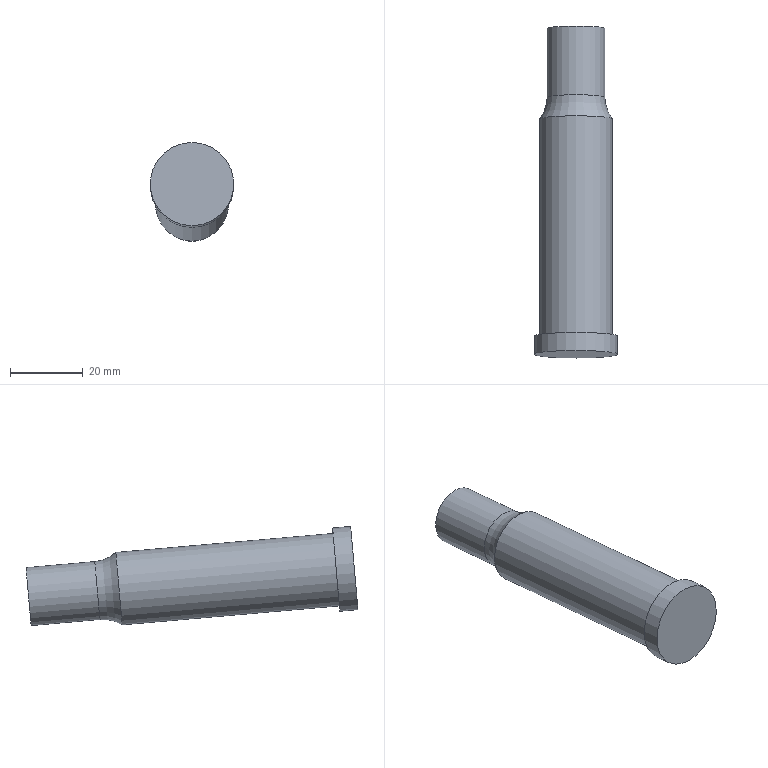Part | NX | features SPAS 20-80-16.00 2 | 1 solid | 7 faces | box 23 x 91.357 x 27.27 mm | volume 26160 mm3 | plane 3 | cylinder 3 | torus 1 | commonest cylinder face diameters 16 x1 20 x1 23 x1
STEP:
#1=CARTESIAN_POINT('',(398.525,-58.243,-48.565));
#2=VERTEX_POINT('',#1);
#3=CARTESIAN_POINT('',(398.525,-57.546,-40.595));
#4=DIRECTION('',(0.,-0.9962,0.08716));
#5=DIRECTION('',(0.,-0.08716,-0.9962));
#6=AXIS2_PLACEMENT_3D('',#3,#4,#5);
#7=CIRCLE('',#6,8.);
#8=EDGE_CURVE('',#2,#2,#7,.T.);
#9=ORIENTED_EDGE('',*,*,#8,.F.);
#10=EDGE_LOOP('',(#9));
#11=FACE_BOUND('',#10,.T.);
#12=CARTESIAN_POINT('',(398.525,-57.546,-40.595));
#13=DIRECTION('',(0.,0.9962,-0.08716));
#14=DIRECTION('',(0.,0.08716,0.9962));
#15=AXIS2_PLACEMENT_3D('',#12,#13,#14);
#16=PLANE('',#15);
#17=ADVANCED_FACE('',(#11),#16,.T.);
#18=CARTESIAN_POINT('',(398.525,-77.171,-46.909));
#19=VERTEX_POINT('',#18);
#20=CARTESIAN_POINT('',(398.525,-76.474,-38.939));
#21=DIRECTION('',(0.,-0.9962,0.08716));
#22=DIRECTION('',(0.,-0.08716,-0.9962));
#23=AXIS2_PLACEMENT_3D('',#20,#21,#22);
#24=CIRCLE('',#23,8.);
#25=EDGE_CURVE('',#19,#19,#24,.F.);
#26=ORIENTED_EDGE('',*,*,#25,.T.);
#27=EDGE_LOOP('',(#26));
#28=FACE_BOUND('',#27,.T.);
#29=ORIENTED_EDGE('',*,*,#8,.T.);
#30=EDGE_LOOP('',(#29));
#31=FACE_BOUND('',#30,.T.);
#32=CARTESIAN_POINT('',(398.525,-57.546,-40.595));
#33=DIRECTION('',(0.,-0.9962,0.08716));
#34=DIRECTION('',(0.,-0.08716,-0.9962));
#35=AXIS2_PLACEMENT_3D('',#32,#33,#34);
#36=CYLINDRICAL_SURFACE('',#35,8.);
#37=ADVANCED_FACE('',(#28,#31),#36,.T.);
#38=CARTESIAN_POINT('',(398.525,-141.351,-23.225));
#39=VERTEX_POINT('',#38);
#40=CARTESIAN_POINT('',(398.525,-142.222,-33.187));
#41=DIRECTION('',(0.,0.9962,-0.08716));
#42=DIRECTION('',(0.,0.08716,0.9962));
#43=AXIS2_PLACEMENT_3D('',#40,#41,#42);
#44=CIRCLE('',#43,10.);
#45=EDGE_CURVE('',#39,#39,#44,.F.);
#46=ORIENTED_EDGE('',*,*,#45,.F.);
#47=EDGE_LOOP('',(#46));
#48=FACE_BOUND('',#47,.T.);
#49=CARTESIAN_POINT('',(398.525,-83.322,-48.378));
#50=VERTEX_POINT('',#49);
#51=CARTESIAN_POINT('',(398.525,-82.451,-38.416));
#52=DIRECTION('',(0.,-0.9962,0.08716));
#53=DIRECTION('',(0.,-0.08716,-0.9962));
#54=AXIS2_PLACEMENT_3D('',#51,#52,#53);
#55=CIRCLE('',#54,10.);
#56=EDGE_CURVE('',#50,#50,#55,.T.);
#57=ORIENTED_EDGE('',*,*,#56,.T.);
#58=EDGE_LOOP('',(#57));
#59=FACE_BOUND('',#58,.T.);
#60=CARTESIAN_POINT('',(398.525,-82.451,-38.416));
#61=DIRECTION('',(0.,-0.9962,0.08716));
#62=DIRECTION('',(0.,-0.08716,-0.9962));
#63=AXIS2_PLACEMENT_3D('',#60,#61,#62);
#64=CYLINDRICAL_SURFACE('',#63,10.);
#65=ADVANCED_FACE('',(#48,#59),#64,.T.);
#66=CARTESIAN_POINT('',(398.525,-148.206,-44.208));
#67=VERTEX_POINT('',#66);
#68=CARTESIAN_POINT('',(398.525,-147.203,-32.751));
#69=DIRECTION('',(0.,-0.9962,0.08716));
#70=DIRECTION('',(0.,-0.08716,-0.9962));
#71=AXIS2_PLACEMENT_3D('',#68,#69,#70);
#72=CIRCLE('',#71,11.5);
#73=EDGE_CURVE('',#67,#67,#72,.F.);
#74=ORIENTED_EDGE('',*,*,#73,.F.);
#75=EDGE_LOOP('',(#74));
#76=FACE_BOUND('',#75,.T.);
#77=CARTESIAN_POINT('',(398.525,-147.203,-32.751));
#78=DIRECTION('',(0.,-0.9962,0.08716));
#79=DIRECTION('',(0.,-0.08716,-0.9962));
#80=AXIS2_PLACEMENT_3D('',#77,#78,#79);
#81=PLANE('',#80);
#82=ADVANCED_FACE('',(#76),#81,.T.);
#83=ORIENTED_EDGE('',*,*,#45,.T.);
#84=EDGE_LOOP('',(#83));
#85=FACE_BOUND('',#84,.T.);
#86=CARTESIAN_POINT('',(398.525,-141.22,-21.731));
#87=VERTEX_POINT('',#86);
#88=CARTESIAN_POINT('',(398.525,-142.222,-33.187));
#89=DIRECTION('',(0.,0.9962,-0.08716));
#90=DIRECTION('',(0.,0.08716,0.9962));
#91=AXIS2_PLACEMENT_3D('',#88,#89,#90);
#92=CIRCLE('',#91,11.5);
#93=EDGE_CURVE('',#87,#87,#92,.F.);
#94=ORIENTED_EDGE('',*,*,#93,.F.);
#95=EDGE_LOOP('',(#94));
#96=FACE_BOUND('',#95,.T.);
#97=CARTESIAN_POINT('',(398.525,-142.222,-33.187));
#98=DIRECTION('',(0.,0.9962,-0.08716));
#99=DIRECTION('',(0.,0.08716,0.9962));
#100=AXIS2_PLACEMENT_3D('',#97,#98,#99);
#101=PLANE('',#100);
#102=ADVANCED_FACE('',(#85,#96),#101,.T.);
#103=ORIENTED_EDGE('',*,*,#73,.T.);
#104=EDGE_LOOP('',(#103));
#105=FACE_BOUND('',#104,.T.);
#106=ORIENTED_EDGE('',*,*,#93,.T.);
#107=EDGE_LOOP('',(#106));
#108=FACE_BOUND('',#107,.T.);
#109=CARTESIAN_POINT('',(398.525,-132.26,-34.059));
#110=DIRECTION('',(0.,-0.9962,0.08716));
#111=DIRECTION('',(0.,-0.08716,-0.9962));
#112=AXIS2_PLACEMENT_3D('',#109,#110,#111);
#113=CYLINDRICAL_SURFACE('',#112,11.5);
#114=ADVANCED_FACE('',(#105,#108),#113,.T.);
#115=ORIENTED_EDGE('',*,*,#25,.F.);
#116=EDGE_LOOP('',(#115));
#117=FACE_BOUND('',#116,.T.);
#118=ORIENTED_EDGE('',*,*,#56,.F.);
#119=EDGE_LOOP('',(#118));
#120=FACE_BOUND('',#119,.T.);
#121=CARTESIAN_POINT('',(398.525,-76.474,-38.939));
#122=DIRECTION('',(0.,-0.9962,0.08716));
#123=DIRECTION('',(0.,-0.08716,-0.9962));
#124=AXIS2_PLACEMENT_3D('',#121,#122,#123);
#125=TOROIDAL_SURFACE('',#124,18.,10.);
#126=ADVANCED_FACE('',(#117,#120),#125,.F.);
#127=CLOSED_SHELL('',(#17,#37,#65,#82,#102,#114,#126));
#128=MANIFOLD_SOLID_BREP('',#127);
#129=(LENGTH_UNIT()NAMED_UNIT(*)SI_UNIT(.MILLI.,.METRE.));
#130=UNCERTAINTY_MEASURE_WITH_UNIT(LENGTH_MEASURE(0.00001),#129,'','');
#131=(NAMED_UNIT(*)PLANE_ANGLE_UNIT()SI_UNIT($,.RADIAN.));
#132=(NAMED_UNIT(*)SI_UNIT($,.STERADIAN.)SOLID_ANGLE_UNIT());
#133=(GEOMETRIC_REPRESENTATION_CONTEXT(3)GLOBAL_UNCERTAINTY_ASSIGNED_CONTEXT((#130))GLOBAL_UNIT_ASSIGNED_CONTEXT((#129,#131,#132))REPRESENTATION_CONTEXT('',''));
#134=ADVANCED_BREP_SHAPE_REPRESENTATION('',(#128),#133);